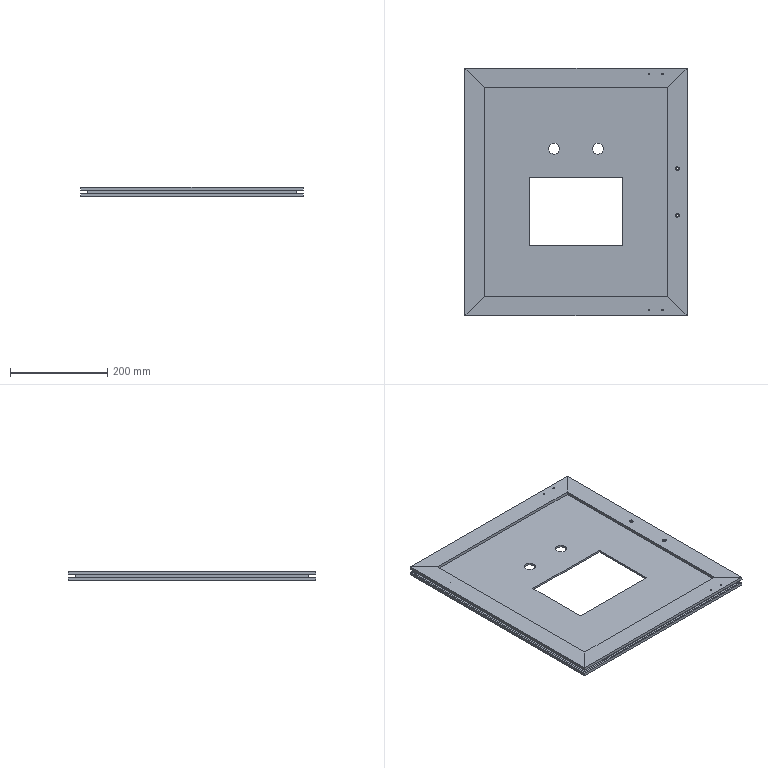Part | SolidWorks | features HoleWzd 3, ICE 3, WeldMemberFeat 1, WeldmentFeature 1 | 5 solids | 192 faces | box 456 x 508 x 20 mm | volume 1433646 mm3 | plane 136 | cylinder 48 | cone 8 | commonest cylinder face diameters 5 x16 3.3 x8 4.5 x8 6.5 x8 8 x4 22.5 x4